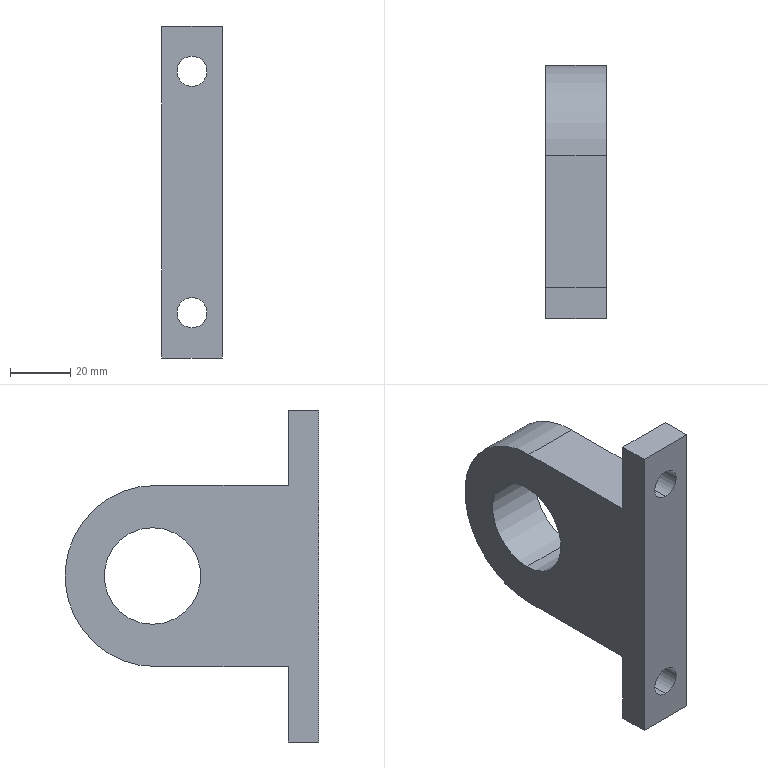Part | SolidWorks | features MoveFace 6, BaseBody 1, DelFace 1, HoleWzd 1, ICE 1, Split 1 | 1 solid | 16 faces | box 20 x 84 x 110 mm | volume 85419 mm3 | plane 9 | cylinder 7 | commonest cylinder face diameters 10 x4 32 x2 60 x1
STEP:
#1=CARTESIAN_POINT('',(-25.,51.,-25.));
#2=VERTEX_POINT('',#1);
#3=CARTESIAN_POINT('',(-25.,51.,-15.));
#4=VERTEX_POINT('',#3);
#5=CARTESIAN_POINT('',(-25.,51.,-20.));
#6=DIRECTION('',(0.,1.,0.));
#7=DIRECTION('',(-1.,0.,0.));
#8=AXIS2_PLACEMENT_3D('',#5,#6,#7);
#9=CIRCLE('',#8,5.);
#10=EDGE_CURVE('',#2,#4,#9,.T.);
#11=ORIENTED_EDGE('',*,*,#10,.F.);
#12=CARTESIAN_POINT('',(-25.,61.,-25.));
#13=VERTEX_POINT('',#12);
#14=CARTESIAN_POINT('',(-25.,10.,-25.));
#15=DIRECTION('',(0.,1.,0.));
#16=VECTOR('',#15,1000.);
#17=LINE('',#14,#16);
#18=EDGE_CURVE('',#2,#13,#17,.T.);
#19=ORIENTED_EDGE('',*,*,#18,.T.);
#20=CARTESIAN_POINT('',(-25.,61.,-15.));
#21=VERTEX_POINT('',#20);
#22=CARTESIAN_POINT('',(-25.,61.,-20.));
#23=DIRECTION('',(0.,1.,0.));
#24=DIRECTION('',(-1.,0.,0.));
#25=AXIS2_PLACEMENT_3D('',#22,#23,#24);
#26=CIRCLE('',#25,5.);
#27=EDGE_CURVE('',#13,#21,#26,.T.);
#28=ORIENTED_EDGE('',*,*,#27,.T.);
#29=CARTESIAN_POINT('',(-25.,10.,-15.));
#30=DIRECTION('',(0.,1.,0.));
#31=VECTOR('',#30,1000.);
#32=LINE('',#29,#31);
#33=EDGE_CURVE('',#4,#21,#32,.T.);
#34=ORIENTED_EDGE('',*,*,#33,.F.);
#35=EDGE_LOOP('',(#11,#19,#28,#34));
#36=FACE_OUTER_BOUND('',#35,.T.);
#37=CARTESIAN_POINT('',(-25.,10.,-20.));
#38=DIRECTION('',(0.,1.,0.));
#39=DIRECTION('',(0.,0.,1.));
#40=AXIS2_PLACEMENT_3D('',#37,#38,#39);
#41=CYLINDRICAL_SURFACE('',#40,5.);
#42=ADVANCED_FACE('',(#36),#41,.F.);
#43=CARTESIAN_POINT('',(-25.,51.,55.));
#44=VERTEX_POINT('',#43);
#45=CARTESIAN_POINT('',(-25.,51.,65.));
#46=VERTEX_POINT('',#45);
#47=CARTESIAN_POINT('',(-25.,51.,60.));
#48=DIRECTION('',(0.,1.,0.));
#49=DIRECTION('',(-1.,0.,0.));
#50=AXIS2_PLACEMENT_3D('',#47,#48,#49);
#51=CIRCLE('',#50,5.);
#52=EDGE_CURVE('',#44,#46,#51,.T.);
#53=ORIENTED_EDGE('',*,*,#52,.F.);
#54=CARTESIAN_POINT('',(-25.,61.,55.));
#55=VERTEX_POINT('',#54);
#56=CARTESIAN_POINT('',(-25.,10.,55.));
#57=DIRECTION('',(0.,1.,0.));
#58=VECTOR('',#57,1000.);
#59=LINE('',#56,#58);
#60=EDGE_CURVE('',#44,#55,#59,.T.);
#61=ORIENTED_EDGE('',*,*,#60,.T.);
#62=CARTESIAN_POINT('',(-25.,61.,65.));
#63=VERTEX_POINT('',#62);
#64=CARTESIAN_POINT('',(-25.,61.,60.));
#65=DIRECTION('',(0.,1.,0.));
#66=DIRECTION('',(-1.,0.,0.));
#67=AXIS2_PLACEMENT_3D('',#64,#65,#66);
#68=CIRCLE('',#67,5.);
#69=EDGE_CURVE('',#55,#63,#68,.T.);
#70=ORIENTED_EDGE('',*,*,#69,.T.);
#71=CARTESIAN_POINT('',(-25.,10.,65.));
#72=DIRECTION('',(0.,1.,0.));
#73=VECTOR('',#72,1000.);
#74=LINE('',#71,#73);
#75=EDGE_CURVE('',#46,#63,#74,.T.);
#76=ORIENTED_EDGE('',*,*,#75,.F.);
#77=EDGE_LOOP('',(#53,#61,#70,#76));
#78=FACE_OUTER_BOUND('',#77,.T.);
#79=CARTESIAN_POINT('',(-25.,10.,60.));
#80=DIRECTION('',(0.,1.,0.));
#81=DIRECTION('',(0.,0.,1.));
#82=AXIS2_PLACEMENT_3D('',#79,#80,#81);
#83=CYLINDRICAL_SURFACE('',#82,5.);
#84=ADVANCED_FACE('',(#78),#83,.F.);
#85=CARTESIAN_POINT('',(-35.,106.,36.));
#86=VERTEX_POINT('',#85);
#87=CARTESIAN_POINT('',(-35.,106.,4.));
#88=VERTEX_POINT('',#87);
#89=CARTESIAN_POINT('',(-35.,106.,20.));
#90=DIRECTION('',(1.,0.,0.));
#91=DIRECTION('',(0.,0.,-1.));
#92=AXIS2_PLACEMENT_3D('',#89,#90,#91);
#93=CIRCLE('',#92,16.);
#94=EDGE_CURVE('',#86,#88,#93,.T.);
#95=ORIENTED_EDGE('',*,*,#94,.F.);
#96=CARTESIAN_POINT('',(-15.,106.,36.));
#97=VERTEX_POINT('',#96);
#98=CARTESIAN_POINT('',(-35.,106.,36.));
#99=DIRECTION('',(1.,0.,0.));
#100=VECTOR('',#99,1000.);
#101=LINE('',#98,#100);
#102=EDGE_CURVE('',#86,#97,#101,.T.);
#103=ORIENTED_EDGE('',*,*,#102,.T.);
#104=CARTESIAN_POINT('',(-15.,106.,4.));
#105=VERTEX_POINT('',#104);
#106=CARTESIAN_POINT('',(-15.,106.,20.));
#107=DIRECTION('',(-1.,0.,0.));
#108=DIRECTION('',(0.,-1.,0.));
#109=AXIS2_PLACEMENT_3D('',#106,#107,#108);
#110=CIRCLE('',#109,16.);
#111=EDGE_CURVE('',#105,#97,#110,.T.);
#112=ORIENTED_EDGE('',*,*,#111,.F.);
#113=CARTESIAN_POINT('',(-35.,106.,4.));
#114=DIRECTION('',(1.,0.,0.));
#115=VECTOR('',#114,1000.);
#116=LINE('',#113,#115);
#117=EDGE_CURVE('',#88,#105,#116,.T.);
#118=ORIENTED_EDGE('',*,*,#117,.F.);
#119=EDGE_LOOP('',(#95,#103,#112,#118));
#120=FACE_OUTER_BOUND('',#119,.T.);
#121=CARTESIAN_POINT('',(-35.,106.,20.));
#122=DIRECTION('',(1.,0.,0.));
#123=DIRECTION('',(0.,0.,-1.));
#124=AXIS2_PLACEMENT_3D('',#121,#122,#123);
#125=CYLINDRICAL_SURFACE('',#124,16.);
#126=ADVANCED_FACE('',(#120),#125,.F.);
#127=CARTESIAN_POINT('',(-25.,51.,-20.));
#128=DIRECTION('',(0.,1.,0.));
#129=DIRECTION('',(-1.,0.,0.));
#130=AXIS2_PLACEMENT_3D('',#127,#128,#129);
#131=CIRCLE('',#130,5.);
#132=EDGE_CURVE('',#4,#2,#131,.T.);
#133=ORIENTED_EDGE('',*,*,#132,.T.);
#134=ORIENTED_EDGE('',*,*,#10,.T.);
#135=EDGE_LOOP('',(#133,#134));
#136=FACE_BOUND('',#135,.T.);
#137=CARTESIAN_POINT('',(-25.,51.,60.));
#138=DIRECTION('',(0.,1.,0.));
#139=DIRECTION('',(-1.,0.,0.));
#140=AXIS2_PLACEMENT_3D('',#137,#138,#139);
#141=CIRCLE('',#140,5.);
#142=EDGE_CURVE('',#46,#44,#141,.T.);
#143=ORIENTED_EDGE('',*,*,#142,.T.);
#144=ORIENTED_EDGE('',*,*,#52,.T.);
#145=EDGE_LOOP('',(#143,#144));
#146=FACE_BOUND('',#145,.T.);
#147=CARTESIAN_POINT('',(-15.,51.,75.));
#148=VERTEX_POINT('',#147);
#149=CARTESIAN_POINT('',(-15.,51.,-35.));
#150=VERTEX_POINT('',#149);
#151=CARTESIAN_POINT('',(-15.,51.,40.));
#152=DIRECTION('',(0.,0.,-1.));
#153=VECTOR('',#152,1000.);
#154=LINE('',#151,#153);
#155=EDGE_CURVE('',#148,#150,#154,.T.);
#156=ORIENTED_EDGE('',*,*,#155,.F.);
#157=CARTESIAN_POINT('',(-35.,51.,75.));
#158=VERTEX_POINT('',#157);
#159=CARTESIAN_POINT('',(-35.,51.,75.));
#160=DIRECTION('',(-1.,0.,0.));
#161=VECTOR('',#160,1000.);
#162=LINE('',#159,#161);
#163=EDGE_CURVE('',#148,#158,#162,.T.);
#164=ORIENTED_EDGE('',*,*,#163,.T.);
#165=CARTESIAN_POINT('',(-35.,51.,-35.));
#166=VERTEX_POINT('',#165);
#167=CARTESIAN_POINT('',(-35.,51.,40.));
#168=DIRECTION('',(0.,0.,-1.));
#169=VECTOR('',#168,1000.);
#170=LINE('',#167,#169);
#171=EDGE_CURVE('',#158,#166,#170,.T.);
#172=ORIENTED_EDGE('',*,*,#171,.T.);
#173=CARTESIAN_POINT('',(-35.,51.,-35.));
#174=DIRECTION('',(1.,0.,0.));
#175=VECTOR('',#174,1000.);
#176=LINE('',#173,#175);
#177=EDGE_CURVE('',#166,#150,#176,.T.);
#178=ORIENTED_EDGE('',*,*,#177,.T.);
#179=EDGE_LOOP('',(#156,#164,#172,#178));
#180=FACE_OUTER_BOUND('',#179,.T.);
#181=CARTESIAN_POINT('',(0.,51.,40.));
#182=DIRECTION('',(0.,1.,0.));
#183=DIRECTION('',(-1.,0.,0.));
#184=AXIS2_PLACEMENT_3D('',#181,#182,#183);
#185=PLANE('',#184);
#186=ADVANCED_FACE('',(#136,#146,#180),#185,.F.);
#187=CARTESIAN_POINT('',(-35.,105.,50.));
#188=VERTEX_POINT('',#187);
#189=CARTESIAN_POINT('',(-35.,61.,50.));
#190=VERTEX_POINT('',#189);
#191=CARTESIAN_POINT('',(-35.,0.,50.));
#192=DIRECTION('',(0.,-1.,0.));
#193=VECTOR('',#192,1000.);
#194=LINE('',#191,#193);
#195=EDGE_CURVE('',#188,#190,#194,.T.);
#196=ORIENTED_EDGE('',*,*,#195,.T.);
#197=CARTESIAN_POINT('',(-15.,61.,50.));
#198=VERTEX_POINT('',#197);
#199=CARTESIAN_POINT('',(0.,61.,50.));
#200=DIRECTION('',(1.,0.,0.));
#201=VECTOR('',#200,1000.);
#202=LINE('',#199,#201);
#203=EDGE_CURVE('',#190,#198,#202,.T.);
#204=ORIENTED_EDGE('',*,*,#203,.T.);
#205=CARTESIAN_POINT('',(-15.,105.,50.));
#206=VERTEX_POINT('',#205);
#207=CARTESIAN_POINT('',(-15.,125.,50.));
#208=DIRECTION('',(0.,-1.,0.));
#209=VECTOR('',#208,1000.);
#210=LINE('',#207,#209);
#211=EDGE_CURVE('',#206,#198,#210,.T.);
#212=ORIENTED_EDGE('',*,*,#211,.F.);
#213=CARTESIAN_POINT('',(0.,105.,50.));
#214=DIRECTION('',(1.,0.,0.));
#215=VECTOR('',#214,1000.);
#216=LINE('',#213,#215);
#217=EDGE_CURVE('',#188,#206,#216,.T.);
#218=ORIENTED_EDGE('',*,*,#217,.F.);
#219=EDGE_LOOP('',(#196,#204,#212,#218));
#220=FACE_OUTER_BOUND('',#219,.T.);
#221=CARTESIAN_POINT('',(0.,0.,50.));
#222=DIRECTION('',(0.,0.,-1.));
#223=DIRECTION('',(-1.,0.,0.));
#224=AXIS2_PLACEMENT_3D('',#221,#222,#223);
#225=PLANE('',#224);
#226=ADVANCED_FACE('',(#220),#225,.F.);
#227=CARTESIAN_POINT('',(-35.,61.,-10.));
#228=VERTEX_POINT('',#227);
#229=CARTESIAN_POINT('',(-35.,105.,-10.));
#230=VERTEX_POINT('',#229);
#231=CARTESIAN_POINT('',(-35.,0.,-10.));
#232=DIRECTION('',(0.,1.,0.));
#233=VECTOR('',#232,1000.);
#234=LINE('',#231,#233);
#235=EDGE_CURVE('',#228,#230,#234,.T.);
#236=ORIENTED_EDGE('',*,*,#235,.F.);
#237=CARTESIAN_POINT('',(-35.,61.,-35.));
#238=VERTEX_POINT('',#237);
#239=CARTESIAN_POINT('',(-35.,61.,0.));
#240=DIRECTION('',(0.,0.,-1.));
#241=VECTOR('',#240,1000.);
#242=LINE('',#239,#241);
#243=EDGE_CURVE('',#228,#238,#242,.T.);
#244=ORIENTED_EDGE('',*,*,#243,.T.);
#245=CARTESIAN_POINT('',(-35.,10.,-35.));
#246=DIRECTION('',(0.,-1.,0.));
#247=VECTOR('',#246,1000.);
#248=LINE('',#245,#247);
#249=EDGE_CURVE('',#238,#166,#248,.T.);
#250=ORIENTED_EDGE('',*,*,#249,.T.);
#251=ORIENTED_EDGE('',*,*,#171,.F.);
#252=CARTESIAN_POINT('',(-35.,61.,75.));
#253=VERTEX_POINT('',#252);
#254=CARTESIAN_POINT('',(-35.,10.,75.));
#255=DIRECTION('',(0.,-1.,0.));
#256=VECTOR('',#255,1000.);
#257=LINE('',#254,#256);
#258=EDGE_CURVE('',#253,#158,#257,.T.);
#259=ORIENTED_EDGE('',*,*,#258,.F.);
#260=CARTESIAN_POINT('',(-35.,61.,0.));
#261=DIRECTION('',(0.,0.,-1.));
#262=VECTOR('',#261,1000.);
#263=LINE('',#260,#262);
#264=EDGE_CURVE('',#253,#190,#263,.T.);
#265=ORIENTED_EDGE('',*,*,#264,.T.);
#266=ORIENTED_EDGE('',*,*,#195,.F.);
#267=CARTESIAN_POINT('',(-35.,105.,20.));
#268=DIRECTION('',(1.,0.,0.));
#269=DIRECTION('',(0.,0.,-1.));
#270=AXIS2_PLACEMENT_3D('',#267,#268,#269);
#271=CIRCLE('',#270,30.);
#272=EDGE_CURVE('',#230,#188,#271,.T.);
#273=ORIENTED_EDGE('',*,*,#272,.F.);
#274=EDGE_LOOP('',(#236,#244,#250,#251,#259,#265,#266,#273));
#275=FACE_OUTER_BOUND('',#274,.T.);
#276=CARTESIAN_POINT('',(-35.,106.,20.));
#277=DIRECTION('',(1.,0.,0.));
#278=DIRECTION('',(0.,0.,-1.));
#279=AXIS2_PLACEMENT_3D('',#276,#277,#278);
#280=CIRCLE('',#279,16.);
#281=EDGE_CURVE('',#88,#86,#280,.T.);
#282=ORIENTED_EDGE('',*,*,#281,.T.);
#283=ORIENTED_EDGE('',*,*,#94,.T.);
#284=EDGE_LOOP('',(#282,#283));
#285=FACE_BOUND('',#284,.T.);
#286=CARTESIAN_POINT('',(-35.,0.,40.));
#287=DIRECTION('',(1.,0.,0.));
#288=DIRECTION('',(0.,0.,-1.));
#289=AXIS2_PLACEMENT_3D('',#286,#287,#288);
#290=PLANE('',#289);
#291=ADVANCED_FACE('',(#275,#285),#290,.F.);
#292=ORIENTED_EDGE('',*,*,#102,.F.);
#293=ORIENTED_EDGE('',*,*,#281,.F.);
#294=ORIENTED_EDGE('',*,*,#117,.T.);
#295=CARTESIAN_POINT('',(-15.,106.,20.));
#296=DIRECTION('',(-1.,0.,0.));
#297=DIRECTION('',(0.,-1.,0.));
#298=AXIS2_PLACEMENT_3D('',#295,#296,#297);
#299=CIRCLE('',#298,16.);
#300=EDGE_CURVE('',#97,#105,#299,.T.);
#301=ORIENTED_EDGE('',*,*,#300,.F.);
#302=EDGE_LOOP('',(#292,#293,#294,#301));
#303=FACE_OUTER_BOUND('',#302,.T.);
#304=CARTESIAN_POINT('',(-35.,106.,20.));
#305=DIRECTION('',(1.,0.,0.));
#306=DIRECTION('',(0.,0.,-1.));
#307=AXIS2_PLACEMENT_3D('',#304,#305,#306);
#308=CYLINDRICAL_SURFACE('',#307,16.);
#309=ADVANCED_FACE('',(#303),#308,.F.);
#310=CARTESIAN_POINT('',(-15.,61.,-10.));
#311=VERTEX_POINT('',#310);
#312=CARTESIAN_POINT('',(0.,61.,-10.));
#313=DIRECTION('',(1.,0.,0.));
#314=VECTOR('',#313,1000.);
#315=LINE('',#312,#314);
#316=EDGE_CURVE('',#228,#311,#315,.T.);
#317=ORIENTED_EDGE('',*,*,#316,.F.);
#318=ORIENTED_EDGE('',*,*,#235,.T.);
#319=CARTESIAN_POINT('',(-15.,105.,-10.));
#320=VERTEX_POINT('',#319);
#321=CARTESIAN_POINT('',(0.,105.,-10.));
#322=DIRECTION('',(-1.,0.,0.));
#323=VECTOR('',#322,1000.);
#324=LINE('',#321,#323);
#325=EDGE_CURVE('',#320,#230,#324,.T.);
#326=ORIENTED_EDGE('',*,*,#325,.F.);
#327=CARTESIAN_POINT('',(-15.,125.,-10.));
#328=DIRECTION('',(0.,-1.,0.));
#329=VECTOR('',#328,1000.);
#330=LINE('',#327,#329);
#331=EDGE_CURVE('',#320,#311,#330,.T.);
#332=ORIENTED_EDGE('',*,*,#331,.T.);
#333=EDGE_LOOP('',(#317,#318,#326,#332));
#334=FACE_OUTER_BOUND('',#333,.T.);
#335=CARTESIAN_POINT('',(0.,0.,-10.));
#336=DIRECTION('',(0.,0.,-1.));
#337=DIRECTION('',(-1.,0.,0.));
#338=AXIS2_PLACEMENT_3D('',#335,#336,#337);
#339=PLANE('',#338);
#340=ADVANCED_FACE('',(#334),#339,.T.);
#341=CARTESIAN_POINT('',(-15.,105.,20.));
#342=DIRECTION('',(-1.,0.,0.));
#343=DIRECTION('',(0.,-1.,0.));
#344=AXIS2_PLACEMENT_3D('',#341,#342,#343);
#345=CIRCLE('',#344,30.);
#346=EDGE_CURVE('',#206,#320,#345,.T.);
#347=ORIENTED_EDGE('',*,*,#346,.T.);
#348=ORIENTED_EDGE('',*,*,#325,.T.);
#349=ORIENTED_EDGE('',*,*,#272,.T.);
#350=ORIENTED_EDGE('',*,*,#217,.T.);
#351=EDGE_LOOP('',(#347,#348,#349,#350));
#352=FACE_OUTER_BOUND('',#351,.T.);
#353=CARTESIAN_POINT('',(0.,105.,20.));
#354=DIRECTION('',(-1.,0.,0.));
#355=DIRECTION('',(0.,0.,1.));
#356=AXIS2_PLACEMENT_3D('',#353,#354,#355);
#357=CYLINDRICAL_SURFACE('',#356,30.);
#358=ADVANCED_FACE('',(#352),#357,.T.);
#359=ORIENTED_EDGE('',*,*,#211,.T.);
#360=CARTESIAN_POINT('',(-15.,61.,75.));
#361=VERTEX_POINT('',#360);
#362=CARTESIAN_POINT('',(-15.,61.,-10.));
#363=DIRECTION('',(0.,0.,1.));
#364=VECTOR('',#363,1000.);
#365=LINE('',#362,#364);
#366=EDGE_CURVE('',#198,#361,#365,.T.);
#367=ORIENTED_EDGE('',*,*,#366,.T.);
#368=CARTESIAN_POINT('',(-15.,10.,75.));
#369=DIRECTION('',(0.,-1.,0.));
#370=VECTOR('',#369,1000.);
#371=LINE('',#368,#370);
#372=EDGE_CURVE('',#361,#148,#371,.T.);
#373=ORIENTED_EDGE('',*,*,#372,.T.);
#374=ORIENTED_EDGE('',*,*,#155,.T.);
#375=CARTESIAN_POINT('',(-15.,61.,-35.));
#376=VERTEX_POINT('',#375);
#377=CARTESIAN_POINT('',(-15.,10.,-35.));
#378=DIRECTION('',(0.,-1.,0.));
#379=VECTOR('',#378,1000.);
#380=LINE('',#377,#379);
#381=EDGE_CURVE('',#376,#150,#380,.T.);
#382=ORIENTED_EDGE('',*,*,#381,.F.);
#383=CARTESIAN_POINT('',(-15.,61.,-10.));
#384=DIRECTION('',(0.,0.,1.));
#385=VECTOR('',#384,1000.);
#386=LINE('',#383,#385);
#387=EDGE_CURVE('',#376,#311,#386,.T.);
#388=ORIENTED_EDGE('',*,*,#387,.T.);
#389=ORIENTED_EDGE('',*,*,#331,.F.);
#390=ORIENTED_EDGE('',*,*,#346,.F.);
#391=EDGE_LOOP('',(#359,#367,#373,#374,#382,#388,#389,#390));
#392=FACE_OUTER_BOUND('',#391,.T.);
#393=ORIENTED_EDGE('',*,*,#111,.T.);
#394=ORIENTED_EDGE('',*,*,#300,.T.);
#395=EDGE_LOOP('',(#393,#394));
#396=FACE_BOUND('',#395,.T.);
#397=CARTESIAN_POINT('',(-15.,105.,-10.));
#398=DIRECTION('',(1.,0.,0.));
#399=DIRECTION('',(0.,1.,0.));
#400=AXIS2_PLACEMENT_3D('',#397,#398,#399);
#401=PLANE('',#400);
#402=ADVANCED_FACE('',(#392,#396),#401,.T.);
#403=ORIENTED_EDGE('',*,*,#177,.F.);
#404=ORIENTED_EDGE('',*,*,#249,.F.);
#405=CARTESIAN_POINT('',(-35.,61.,-35.));
#406=DIRECTION('',(1.,0.,0.));
#407=VECTOR('',#406,1000.);
#408=LINE('',#405,#407);
#409=EDGE_CURVE('',#238,#376,#408,.T.);
#410=ORIENTED_EDGE('',*,*,#409,.T.);
#411=ORIENTED_EDGE('',*,*,#381,.T.);
#412=EDGE_LOOP('',(#403,#404,#410,#411));
#413=FACE_OUTER_BOUND('',#412,.T.);
#414=CARTESIAN_POINT('',(-35.,10.,-35.));
#415=DIRECTION('',(0.,0.,-1.));
#416=DIRECTION('',(-1.,0.,0.));
#417=AXIS2_PLACEMENT_3D('',#414,#415,#416);
#418=PLANE('',#417);
#419=ADVANCED_FACE('',(#413),#418,.T.);
#420=CARTESIAN_POINT('',(-25.,61.,-20.));
#421=DIRECTION('',(0.,1.,0.));
#422=DIRECTION('',(-1.,0.,0.));
#423=AXIS2_PLACEMENT_3D('',#420,#421,#422);
#424=CIRCLE('',#423,5.);
#425=EDGE_CURVE('',#21,#13,#424,.T.);
#426=ORIENTED_EDGE('',*,*,#425,.F.);
#427=ORIENTED_EDGE('',*,*,#27,.F.);
#428=EDGE_LOOP('',(#426,#427));
#429=FACE_BOUND('',#428,.T.);
#430=ORIENTED_EDGE('',*,*,#243,.F.);
#431=ORIENTED_EDGE('',*,*,#316,.T.);
#432=ORIENTED_EDGE('',*,*,#387,.F.);
#433=ORIENTED_EDGE('',*,*,#409,.F.);
#434=EDGE_LOOP('',(#430,#431,#432,#433));
#435=FACE_OUTER_BOUND('',#434,.T.);
#436=CARTESIAN_POINT('',(0.,61.,0.));
#437=DIRECTION('',(0.,1.,0.));
#438=DIRECTION('',(-1.,0.,0.));
#439=AXIS2_PLACEMENT_3D('',#436,#437,#438);
#440=PLANE('',#439);
#441=ADVANCED_FACE('',(#429,#435),#440,.T.);
#442=CARTESIAN_POINT('',(-25.,61.,60.));
#443=DIRECTION('',(0.,1.,0.));
#444=DIRECTION('',(-1.,0.,0.));
#445=AXIS2_PLACEMENT_3D('',#442,#443,#444);
#446=CIRCLE('',#445,5.);
#447=EDGE_CURVE('',#63,#55,#446,.T.);
#448=ORIENTED_EDGE('',*,*,#447,.F.);
#449=ORIENTED_EDGE('',*,*,#69,.F.);
#450=EDGE_LOOP('',(#448,#449));
#451=FACE_BOUND('',#450,.T.);
#452=ORIENTED_EDGE('',*,*,#203,.F.);
#453=ORIENTED_EDGE('',*,*,#264,.F.);
#454=CARTESIAN_POINT('',(-35.,61.,75.));
#455=DIRECTION('',(-1.,0.,0.));
#456=VECTOR('',#455,1000.);
#457=LINE('',#454,#456);
#458=EDGE_CURVE('',#361,#253,#457,.T.);
#459=ORIENTED_EDGE('',*,*,#458,.F.);
#460=ORIENTED_EDGE('',*,*,#366,.F.);
#461=EDGE_LOOP('',(#452,#453,#459,#460));
#462=FACE_OUTER_BOUND('',#461,.T.);
#463=CARTESIAN_POINT('',(0.,61.,0.));
#464=DIRECTION('',(0.,1.,0.));
#465=DIRECTION('',(-1.,0.,0.));
#466=AXIS2_PLACEMENT_3D('',#463,#464,#465);
#467=PLANE('',#466);
#468=ADVANCED_FACE('',(#451,#462),#467,.T.);
#469=ORIENTED_EDGE('',*,*,#163,.F.);
#470=ORIENTED_EDGE('',*,*,#372,.F.);
#471=ORIENTED_EDGE('',*,*,#458,.T.);
#472=ORIENTED_EDGE('',*,*,#258,.T.);
#473=EDGE_LOOP('',(#469,#470,#471,#472));
#474=FACE_OUTER_BOUND('',#473,.T.);
#475=CARTESIAN_POINT('',(-35.,10.,75.));
#476=DIRECTION('',(0.,0.,1.));
#477=DIRECTION('',(1.,0.,0.));
#478=AXIS2_PLACEMENT_3D('',#475,#476,#477);
#479=PLANE('',#478);
#480=ADVANCED_FACE('',(#474),#479,.T.);
#481=ORIENTED_EDGE('',*,*,#60,.F.);
#482=ORIENTED_EDGE('',*,*,#142,.F.);
#483=ORIENTED_EDGE('',*,*,#75,.T.);
#484=ORIENTED_EDGE('',*,*,#447,.T.);
#485=EDGE_LOOP('',(#481,#482,#483,#484));
#486=FACE_OUTER_BOUND('',#485,.T.);
#487=CARTESIAN_POINT('',(-25.,10.,60.));
#488=DIRECTION('',(0.,1.,0.));
#489=DIRECTION('',(0.,0.,1.));
#490=AXIS2_PLACEMENT_3D('',#487,#488,#489);
#491=CYLINDRICAL_SURFACE('',#490,5.);
#492=ADVANCED_FACE('',(#486),#491,.F.);
#493=ORIENTED_EDGE('',*,*,#18,.F.);
#494=ORIENTED_EDGE('',*,*,#132,.F.);
#495=ORIENTED_EDGE('',*,*,#33,.T.);
#496=ORIENTED_EDGE('',*,*,#425,.T.);
#497=EDGE_LOOP('',(#493,#494,#495,#496));
#498=FACE_OUTER_BOUND('',#497,.T.);
#499=CARTESIAN_POINT('',(-25.,10.,-20.));
#500=DIRECTION('',(0.,1.,0.));
#501=DIRECTION('',(0.,0.,1.));
#502=AXIS2_PLACEMENT_3D('',#499,#500,#501);
#503=CYLINDRICAL_SURFACE('',#502,5.);
#504=ADVANCED_FACE('',(#498),#503,.F.);
#505=CLOSED_SHELL('',(#42,#84,#126,#186,#226,#291,#309,#340,#358,#402,#419,#441,#468,#480,#492,#504));
#506=MANIFOLD_SOLID_BREP('',#505);
#507=CARTESIAN_POINT('',(0.,0.,0.));
#508=DIRECTION('',(0.,0.,1.));
#509=DIRECTION('',(1.,0.,0.));
#510=AXIS2_PLACEMENT_3D('',#507,#508,#509);
#511=(LENGTH_UNIT()NAMED_UNIT(*)SI_UNIT(.MILLI.,.METRE.));
#512=UNCERTAINTY_MEASURE_WITH_UNIT(LENGTH_MEASURE(0.00001),#511,'','');
#513=(NAMED_UNIT(*)PLANE_ANGLE_UNIT()SI_UNIT($,.RADIAN.));
#514=(NAMED_UNIT(*)SI_UNIT($,.STERADIAN.)SOLID_ANGLE_UNIT());
#515=(GEOMETRIC_REPRESENTATION_CONTEXT(3)GLOBAL_UNCERTAINTY_ASSIGNED_CONTEXT((#512))GLOBAL_UNIT_ASSIGNED_CONTEXT((#511,#513,#514))REPRESENTATION_CONTEXT('',''));
#516=ADVANCED_BREP_SHAPE_REPRESENTATION('',(#506,#510),#515);